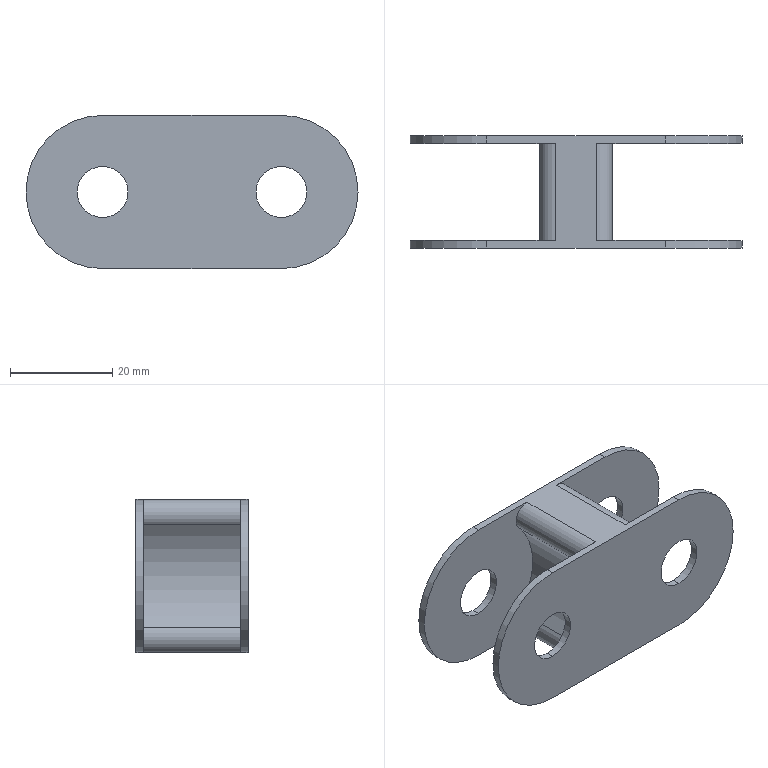Part | SolidWorks | features Extrusion 1, Fillet 1, ICE 1 | 1 solid | 26 faces | box 65 x 22 x 30 mm | volume 10120 mm3 | cylinder 18 | plane 8 | commonest cylinder face diameters 10 x8 30 x6 6 x4
STEP:
#1=CARTESIAN_POINT('',(-17.5,9.5,5.));
#2=VERTEX_POINT('',#1);
#3=CARTESIAN_POINT('',(-17.5,9.5,-5.));
#4=VERTEX_POINT('',#3);
#5=CARTESIAN_POINT('',(-17.5,9.5,0.));
#6=DIRECTION('',(0.,-1.,0.));
#7=DIRECTION('',(0.,0.,1.));
#8=AXIS2_PLACEMENT_3D('',#5,#6,#7);
#9=CIRCLE('',#8,5.);
#10=EDGE_CURVE('',#2,#4,#9,.T.);
#11=ORIENTED_EDGE('',*,*,#10,.T.);
#12=CARTESIAN_POINT('',(-17.5,11.,-5.));
#13=VERTEX_POINT('',#12);
#14=CARTESIAN_POINT('',(-17.5,-11.,-5.));
#15=DIRECTION('',(0.,1.,0.));
#16=VECTOR('',#15,1000.);
#17=LINE('',#14,#16);
#18=EDGE_CURVE('',#4,#13,#17,.T.);
#19=ORIENTED_EDGE('',*,*,#18,.T.);
#20=CARTESIAN_POINT('',(-17.5,11.,5.));
#21=VERTEX_POINT('',#20);
#22=CARTESIAN_POINT('',(-17.5,11.,0.));
#23=DIRECTION('',(0.,1.,0.));
#24=DIRECTION('',(0.,0.,1.));
#25=AXIS2_PLACEMENT_3D('',#22,#23,#24);
#26=CIRCLE('',#25,5.);
#27=EDGE_CURVE('',#13,#21,#26,.T.);
#28=ORIENTED_EDGE('',*,*,#27,.T.);
#29=CARTESIAN_POINT('',(-17.5,-11.,5.));
#30=DIRECTION('',(0.,1.,0.));
#31=VECTOR('',#30,1000.);
#32=LINE('',#29,#31);
#33=EDGE_CURVE('',#2,#21,#32,.T.);
#34=ORIENTED_EDGE('',*,*,#33,.F.);
#35=EDGE_LOOP('',(#11,#19,#28,#34));
#36=FACE_OUTER_BOUND('',#35,.T.);
#37=CARTESIAN_POINT('',(-17.5,-11.,0.));
#38=DIRECTION('',(0.,1.,0.));
#39=DIRECTION('',(0.,0.,1.));
#40=AXIS2_PLACEMENT_3D('',#37,#38,#39);
#41=CYLINDRICAL_SURFACE('',#40,5.);
#42=ADVANCED_FACE('',(#36),#41,.F.);
#43=CARTESIAN_POINT('',(17.5,9.5,5.));
#44=VERTEX_POINT('',#43);
#45=CARTESIAN_POINT('',(17.5,9.5,-5.));
#46=VERTEX_POINT('',#45);
#47=CARTESIAN_POINT('',(17.5,9.5,0.));
#48=DIRECTION('',(0.,-1.,0.));
#49=DIRECTION('',(0.,0.,1.));
#50=AXIS2_PLACEMENT_3D('',#47,#48,#49);
#51=CIRCLE('',#50,5.);
#52=EDGE_CURVE('',#44,#46,#51,.T.);
#53=ORIENTED_EDGE('',*,*,#52,.T.);
#54=CARTESIAN_POINT('',(17.5,11.,-5.));
#55=VERTEX_POINT('',#54);
#56=CARTESIAN_POINT('',(17.5,-11.,-5.));
#57=DIRECTION('',(0.,1.,0.));
#58=VECTOR('',#57,1000.);
#59=LINE('',#56,#58);
#60=EDGE_CURVE('',#46,#55,#59,.T.);
#61=ORIENTED_EDGE('',*,*,#60,.T.);
#62=CARTESIAN_POINT('',(17.5,11.,5.));
#63=VERTEX_POINT('',#62);
#64=CARTESIAN_POINT('',(17.5,11.,0.));
#65=DIRECTION('',(0.,1.,0.));
#66=DIRECTION('',(0.,0.,1.));
#67=AXIS2_PLACEMENT_3D('',#64,#65,#66);
#68=CIRCLE('',#67,5.);
#69=EDGE_CURVE('',#55,#63,#68,.T.);
#70=ORIENTED_EDGE('',*,*,#69,.T.);
#71=CARTESIAN_POINT('',(17.5,-11.,5.));
#72=DIRECTION('',(0.,1.,0.));
#73=VECTOR('',#72,1000.);
#74=LINE('',#71,#73);
#75=EDGE_CURVE('',#44,#63,#74,.T.);
#76=ORIENTED_EDGE('',*,*,#75,.F.);
#77=EDGE_LOOP('',(#53,#61,#70,#76));
#78=FACE_OUTER_BOUND('',#77,.T.);
#79=CARTESIAN_POINT('',(17.5,-11.,0.));
#80=DIRECTION('',(0.,1.,0.));
#81=DIRECTION('',(0.,0.,1.));
#82=AXIS2_PLACEMENT_3D('',#79,#80,#81);
#83=CYLINDRICAL_SURFACE('',#82,5.);
#84=ADVANCED_FACE('',(#78),#83,.F.);
#85=CARTESIAN_POINT('',(-17.5,-11.,-5.));
#86=VERTEX_POINT('',#85);
#87=CARTESIAN_POINT('',(-17.5,-11.,5.));
#88=VERTEX_POINT('',#87);
#89=CARTESIAN_POINT('',(-17.5,-11.,0.));
#90=DIRECTION('',(0.,1.,0.));
#91=DIRECTION('',(0.,0.,1.));
#92=AXIS2_PLACEMENT_3D('',#89,#90,#91);
#93=CIRCLE('',#92,5.);
#94=EDGE_CURVE('',#86,#88,#93,.T.);
#95=ORIENTED_EDGE('',*,*,#94,.F.);
#96=CARTESIAN_POINT('',(-17.5,-9.5,-5.));
#97=VERTEX_POINT('',#96);
#98=CARTESIAN_POINT('',(-17.5,-11.,-5.));
#99=DIRECTION('',(0.,1.,0.));
#100=VECTOR('',#99,1000.);
#101=LINE('',#98,#100);
#102=EDGE_CURVE('',#86,#97,#101,.T.);
#103=ORIENTED_EDGE('',*,*,#102,.T.);
#104=CARTESIAN_POINT('',(-17.5,-9.5,5.));
#105=VERTEX_POINT('',#104);
#106=CARTESIAN_POINT('',(-17.5,-9.5,0.));
#107=DIRECTION('',(0.,-1.,0.));
#108=DIRECTION('',(0.,0.,1.));
#109=AXIS2_PLACEMENT_3D('',#106,#107,#108);
#110=CIRCLE('',#109,5.);
#111=EDGE_CURVE('',#105,#97,#110,.T.);
#112=ORIENTED_EDGE('',*,*,#111,.F.);
#113=CARTESIAN_POINT('',(-17.5,-11.,5.));
#114=DIRECTION('',(0.,1.,0.));
#115=VECTOR('',#114,1000.);
#116=LINE('',#113,#115);
#117=EDGE_CURVE('',#88,#105,#116,.T.);
#118=ORIENTED_EDGE('',*,*,#117,.F.);
#119=EDGE_LOOP('',(#95,#103,#112,#118));
#120=FACE_OUTER_BOUND('',#119,.T.);
#121=CARTESIAN_POINT('',(-17.5,-11.,0.));
#122=DIRECTION('',(0.,1.,0.));
#123=DIRECTION('',(0.,0.,1.));
#124=AXIS2_PLACEMENT_3D('',#121,#122,#123);
#125=CYLINDRICAL_SURFACE('',#124,5.);
#126=ADVANCED_FACE('',(#120),#125,.F.);
#127=CARTESIAN_POINT('',(17.5,-11.,-5.));
#128=VERTEX_POINT('',#127);
#129=CARTESIAN_POINT('',(17.5,-11.,5.));
#130=VERTEX_POINT('',#129);
#131=CARTESIAN_POINT('',(17.5,-11.,0.));
#132=DIRECTION('',(0.,1.,0.));
#133=DIRECTION('',(0.,0.,1.));
#134=AXIS2_PLACEMENT_3D('',#131,#132,#133);
#135=CIRCLE('',#134,5.);
#136=EDGE_CURVE('',#128,#130,#135,.T.);
#137=ORIENTED_EDGE('',*,*,#136,.F.);
#138=CARTESIAN_POINT('',(17.5,-9.5,-5.));
#139=VERTEX_POINT('',#138);
#140=CARTESIAN_POINT('',(17.5,-11.,-5.));
#141=DIRECTION('',(0.,1.,0.));
#142=VECTOR('',#141,1000.);
#143=LINE('',#140,#142);
#144=EDGE_CURVE('',#128,#139,#143,.T.);
#145=ORIENTED_EDGE('',*,*,#144,.T.);
#146=CARTESIAN_POINT('',(17.5,-9.5,5.));
#147=VERTEX_POINT('',#146);
#148=CARTESIAN_POINT('',(17.5,-9.5,0.));
#149=DIRECTION('',(0.,-1.,0.));
#150=DIRECTION('',(0.,0.,1.));
#151=AXIS2_PLACEMENT_3D('',#148,#149,#150);
#152=CIRCLE('',#151,5.);
#153=EDGE_CURVE('',#147,#139,#152,.T.);
#154=ORIENTED_EDGE('',*,*,#153,.F.);
#155=CARTESIAN_POINT('',(17.5,-11.,5.));
#156=DIRECTION('',(0.,1.,0.));
#157=VECTOR('',#156,1000.);
#158=LINE('',#155,#157);
#159=EDGE_CURVE('',#130,#147,#158,.T.);
#160=ORIENTED_EDGE('',*,*,#159,.F.);
#161=EDGE_LOOP('',(#137,#145,#154,#160));
#162=FACE_OUTER_BOUND('',#161,.T.);
#163=CARTESIAN_POINT('',(17.5,-11.,0.));
#164=DIRECTION('',(0.,1.,0.));
#165=DIRECTION('',(0.,0.,1.));
#166=AXIS2_PLACEMENT_3D('',#163,#164,#165);
#167=CYLINDRICAL_SURFACE('',#166,5.);
#168=ADVANCED_FACE('',(#162),#167,.F.);
#169=CARTESIAN_POINT('',(17.5,-11.,-15.));
#170=VERTEX_POINT('',#169);
#171=CARTESIAN_POINT('',(17.5,-9.5,-15.));
#172=VERTEX_POINT('',#171);
#173=CARTESIAN_POINT('',(17.5,-11.,-15.));
#174=DIRECTION('',(0.,1.,0.));
#175=VECTOR('',#174,1000.);
#176=LINE('',#173,#175);
#177=EDGE_CURVE('',#170,#172,#176,.T.);
#178=ORIENTED_EDGE('',*,*,#177,.T.);
#179=CARTESIAN_POINT('',(17.5,-9.5,15.));
#180=VERTEX_POINT('',#179);
#181=CARTESIAN_POINT('',(17.5,-9.5,0.));
#182=DIRECTION('',(0.,1.,0.));
#183=DIRECTION('',(0.,0.,1.));
#184=AXIS2_PLACEMENT_3D('',#181,#182,#183);
#185=CIRCLE('',#184,15.);
#186=EDGE_CURVE('',#180,#172,#185,.T.);
#187=ORIENTED_EDGE('',*,*,#186,.F.);
#188=CARTESIAN_POINT('',(17.5,-11.,15.));
#189=VERTEX_POINT('',#188);
#190=CARTESIAN_POINT('',(17.5,-11.,15.));
#191=DIRECTION('',(0.,1.,0.));
#192=VECTOR('',#191,1000.);
#193=LINE('',#190,#192);
#194=EDGE_CURVE('',#189,#180,#193,.T.);
#195=ORIENTED_EDGE('',*,*,#194,.F.);
#196=CARTESIAN_POINT('',(17.5,-11.,0.));
#197=DIRECTION('',(0.,1.,0.));
#198=DIRECTION('',(0.,0.,1.));
#199=AXIS2_PLACEMENT_3D('',#196,#197,#198);
#200=CIRCLE('',#199,15.);
#201=EDGE_CURVE('',#189,#170,#200,.T.);
#202=ORIENTED_EDGE('',*,*,#201,.T.);
#203=EDGE_LOOP('',(#178,#187,#195,#202));
#204=FACE_OUTER_BOUND('',#203,.T.);
#205=CARTESIAN_POINT('',(17.5,-11.,0.));
#206=DIRECTION('',(0.,1.,0.));
#207=DIRECTION('',(0.,0.,1.));
#208=AXIS2_PLACEMENT_3D('',#205,#206,#207);
#209=CYLINDRICAL_SURFACE('',#208,15.);
#210=ADVANCED_FACE('',(#204),#209,.T.);
#211=ORIENTED_EDGE('',*,*,#144,.F.);
#212=CARTESIAN_POINT('',(17.5,-11.,0.));
#213=DIRECTION('',(0.,1.,0.));
#214=DIRECTION('',(0.,0.,1.));
#215=AXIS2_PLACEMENT_3D('',#212,#213,#214);
#216=CIRCLE('',#215,5.);
#217=EDGE_CURVE('',#130,#128,#216,.T.);
#218=ORIENTED_EDGE('',*,*,#217,.F.);
#219=ORIENTED_EDGE('',*,*,#159,.T.);
#220=CARTESIAN_POINT('',(17.5,-9.5,0.));
#221=DIRECTION('',(0.,-1.,0.));
#222=DIRECTION('',(0.,0.,1.));
#223=AXIS2_PLACEMENT_3D('',#220,#221,#222);
#224=CIRCLE('',#223,5.);
#225=EDGE_CURVE('',#139,#147,#224,.T.);
#226=ORIENTED_EDGE('',*,*,#225,.F.);
#227=EDGE_LOOP('',(#211,#218,#219,#226));
#228=FACE_OUTER_BOUND('',#227,.T.);
#229=CARTESIAN_POINT('',(17.5,-11.,0.));
#230=DIRECTION('',(0.,1.,0.));
#231=DIRECTION('',(0.,0.,1.));
#232=AXIS2_PLACEMENT_3D('',#229,#230,#231);
#233=CYLINDRICAL_SURFACE('',#232,5.);
#234=ADVANCED_FACE('',(#228),#233,.F.);
#235=CARTESIAN_POINT('',(-17.5,-11.,15.));
#236=VERTEX_POINT('',#235);
#237=CARTESIAN_POINT('',(-17.5,-9.5,15.));
#238=VERTEX_POINT('',#237);
#239=CARTESIAN_POINT('',(-17.5,-11.,15.));
#240=DIRECTION('',(0.,1.,0.));
#241=VECTOR('',#240,1000.);
#242=LINE('',#239,#241);
#243=EDGE_CURVE('',#236,#238,#242,.T.);
#244=ORIENTED_EDGE('',*,*,#243,.T.);
#245=CARTESIAN_POINT('',(-17.5,-9.5,-15.));
#246=VERTEX_POINT('',#245);
#247=CARTESIAN_POINT('',(-17.5,-9.5,0.));
#248=DIRECTION('',(0.,1.,0.));
#249=DIRECTION('',(0.,0.,1.));
#250=AXIS2_PLACEMENT_3D('',#247,#248,#249);
#251=CIRCLE('',#250,15.);
#252=EDGE_CURVE('',#246,#238,#251,.T.);
#253=ORIENTED_EDGE('',*,*,#252,.F.);
#254=CARTESIAN_POINT('',(-17.5,-11.,-15.));
#255=VERTEX_POINT('',#254);
#256=CARTESIAN_POINT('',(-17.5,-11.,-15.));
#257=DIRECTION('',(0.,1.,0.));
#258=VECTOR('',#257,1000.);
#259=LINE('',#256,#258);
#260=EDGE_CURVE('',#255,#246,#259,.T.);
#261=ORIENTED_EDGE('',*,*,#260,.F.);
#262=CARTESIAN_POINT('',(-17.5,-11.,0.));
#263=DIRECTION('',(0.,1.,0.));
#264=DIRECTION('',(0.,0.,1.));
#265=AXIS2_PLACEMENT_3D('',#262,#263,#264);
#266=CIRCLE('',#265,15.);
#267=EDGE_CURVE('',#255,#236,#266,.T.);
#268=ORIENTED_EDGE('',*,*,#267,.T.);
#269=EDGE_LOOP('',(#244,#253,#261,#268));
#270=FACE_OUTER_BOUND('',#269,.T.);
#271=CARTESIAN_POINT('',(-17.5,-11.,0.));
#272=DIRECTION('',(0.,1.,0.));
#273=DIRECTION('',(0.,0.,1.));
#274=AXIS2_PLACEMENT_3D('',#271,#272,#273);
#275=CYLINDRICAL_SURFACE('',#274,15.);
#276=ADVANCED_FACE('',(#270),#275,.T.);
#277=ORIENTED_EDGE('',*,*,#102,.F.);
#278=CARTESIAN_POINT('',(-17.5,-11.,0.));
#279=DIRECTION('',(0.,1.,0.));
#280=DIRECTION('',(0.,0.,1.));
#281=AXIS2_PLACEMENT_3D('',#278,#279,#280);
#282=CIRCLE('',#281,5.);
#283=EDGE_CURVE('',#88,#86,#282,.T.);
#284=ORIENTED_EDGE('',*,*,#283,.F.);
#285=ORIENTED_EDGE('',*,*,#117,.T.);
#286=CARTESIAN_POINT('',(-17.5,-9.5,0.));
#287=DIRECTION('',(0.,-1.,0.));
#288=DIRECTION('',(0.,0.,1.));
#289=AXIS2_PLACEMENT_3D('',#286,#287,#288);
#290=CIRCLE('',#289,5.);
#291=EDGE_CURVE('',#97,#105,#290,.T.);
#292=ORIENTED_EDGE('',*,*,#291,.F.);
#293=EDGE_LOOP('',(#277,#284,#285,#292));
#294=FACE_OUTER_BOUND('',#293,.T.);
#295=CARTESIAN_POINT('',(-17.5,-11.,0.));
#296=DIRECTION('',(0.,1.,0.));
#297=DIRECTION('',(0.,0.,1.));
#298=AXIS2_PLACEMENT_3D('',#295,#296,#297);
#299=CYLINDRICAL_SURFACE('',#298,5.);
#300=ADVANCED_FACE('',(#294),#299,.F.);
#301=CARTESIAN_POINT('',(-17.5,9.5,-15.));
#302=VERTEX_POINT('',#301);
#303=CARTESIAN_POINT('',(-17.5,9.5,15.));
#304=VERTEX_POINT('',#303);
#305=CARTESIAN_POINT('',(-17.5,9.5,0.));
#306=DIRECTION('',(0.,1.,0.));
#307=DIRECTION('',(0.,0.,1.));
#308=AXIS2_PLACEMENT_3D('',#305,#306,#307);
#309=CIRCLE('',#308,15.);
#310=EDGE_CURVE('',#302,#304,#309,.T.);
#311=ORIENTED_EDGE('',*,*,#310,.T.);
#312=CARTESIAN_POINT('',(-17.5,11.,15.));
#313=VERTEX_POINT('',#312);
#314=CARTESIAN_POINT('',(-17.5,-11.,15.));
#315=DIRECTION('',(0.,1.,0.));
#316=VECTOR('',#315,1000.);
#317=LINE('',#314,#316);
#318=EDGE_CURVE('',#304,#313,#317,.T.);
#319=ORIENTED_EDGE('',*,*,#318,.T.);
#320=CARTESIAN_POINT('',(-17.5,11.,-15.));
#321=VERTEX_POINT('',#320);
#322=CARTESIAN_POINT('',(-17.5,11.,0.));
#323=DIRECTION('',(0.,1.,0.));
#324=DIRECTION('',(0.,0.,1.));
#325=AXIS2_PLACEMENT_3D('',#322,#323,#324);
#326=CIRCLE('',#325,15.);
#327=EDGE_CURVE('',#321,#313,#326,.T.);
#328=ORIENTED_EDGE('',*,*,#327,.F.);
#329=CARTESIAN_POINT('',(-17.5,-11.,-15.));
#330=DIRECTION('',(0.,1.,0.));
#331=VECTOR('',#330,1000.);
#332=LINE('',#329,#331);
#333=EDGE_CURVE('',#302,#321,#332,.T.);
#334=ORIENTED_EDGE('',*,*,#333,.F.);
#335=EDGE_LOOP('',(#311,#319,#328,#334));
#336=FACE_OUTER_BOUND('',#335,.T.);
#337=CARTESIAN_POINT('',(-17.5,-11.,0.));
#338=DIRECTION('',(0.,1.,0.));
#339=DIRECTION('',(0.,0.,1.));
#340=AXIS2_PLACEMENT_3D('',#337,#338,#339);
#341=CYLINDRICAL_SURFACE('',#340,15.);
#342=ADVANCED_FACE('',(#336),#341,.T.);
#343=CARTESIAN_POINT('',(-4.084,-9.5,-15.));
#344=VERTEX_POINT('',#343);
#345=CARTESIAN_POINT('',(-4.084,9.5,-15.));
#346=VERTEX_POINT('',#345);
#347=CARTESIAN_POINT('',(-4.084,-11.,-15.));
#348=DIRECTION('',(0.,1.,0.));
#349=VECTOR('',#348,1000.);
#350=LINE('',#347,#349);
#351=EDGE_CURVE('',#344,#346,#350,.T.);
#352=ORIENTED_EDGE('',*,*,#351,.T.);
#353=CARTESIAN_POINT('',(-17.5,9.5,-15.));
#354=DIRECTION('',(-1.,0.,0.));
#355=VECTOR('',#354,1000.);
#356=LINE('',#353,#355);
#357=EDGE_CURVE('',#346,#302,#356,.T.);
#358=ORIENTED_EDGE('',*,*,#357,.T.);
#359=ORIENTED_EDGE('',*,*,#333,.T.);
#360=CARTESIAN_POINT('',(17.5,11.,-15.));
#361=VERTEX_POINT('',#360);
#362=CARTESIAN_POINT('',(-17.5,11.,-15.));
#363=DIRECTION('',(-1.,0.,0.));
#364=VECTOR('',#363,1000.);
#365=LINE('',#362,#364);
#366=EDGE_CURVE('',#361,#321,#365,.T.);
#367=ORIENTED_EDGE('',*,*,#366,.F.);
#368=CARTESIAN_POINT('',(17.5,9.5,-15.));
#369=VERTEX_POINT('',#368);
#370=CARTESIAN_POINT('',(17.5,-11.,-15.));
#371=DIRECTION('',(0.,1.,0.));
#372=VECTOR('',#371,1000.);
#373=LINE('',#370,#372);
#374=EDGE_CURVE('',#369,#361,#373,.T.);
#375=ORIENTED_EDGE('',*,*,#374,.F.);
#376=CARTESIAN_POINT('',(4.084,9.5,-15.));
#377=VERTEX_POINT('',#376);
#378=CARTESIAN_POINT('',(17.5,9.5,-15.));
#379=DIRECTION('',(-1.,0.,0.));
#380=VECTOR('',#379,1000.);
#381=LINE('',#378,#380);
#382=EDGE_CURVE('',#369,#377,#381,.T.);
#383=ORIENTED_EDGE('',*,*,#382,.T.);
#384=CARTESIAN_POINT('',(4.084,-9.5,-15.));
#385=VERTEX_POINT('',#384);
#386=CARTESIAN_POINT('',(4.084,-11.,-15.));
#387=DIRECTION('',(0.,-1.,0.));
#388=VECTOR('',#387,1000.);
#389=LINE('',#386,#388);
#390=EDGE_CURVE('',#377,#385,#389,.T.);
#391=ORIENTED_EDGE('',*,*,#390,.T.);
#392=CARTESIAN_POINT('',(-17.5,-9.5,-15.));
#393=DIRECTION('',(1.,0.,0.));
#394=VECTOR('',#393,1000.);
#395=LINE('',#392,#394);
#396=EDGE_CURVE('',#385,#172,#395,.T.);
#397=ORIENTED_EDGE('',*,*,#396,.T.);
#398=ORIENTED_EDGE('',*,*,#177,.F.);
#399=CARTESIAN_POINT('',(-17.5,-11.,-15.));
#400=DIRECTION('',(-1.,0.,0.));
#401=VECTOR('',#400,1000.);
#402=LINE('',#399,#401);
#403=EDGE_CURVE('',#170,#255,#402,.T.);
#404=ORIENTED_EDGE('',*,*,#403,.T.);
#405=ORIENTED_EDGE('',*,*,#260,.T.);
#406=CARTESIAN_POINT('',(-17.5,-9.5,-15.));
#407=DIRECTION('',(1.,0.,0.));
#408=VECTOR('',#407,1000.);
#409=LINE('',#406,#408);
#410=EDGE_CURVE('',#246,#344,#409,.T.);
#411=ORIENTED_EDGE('',*,*,#410,.T.);
#412=EDGE_LOOP('',(#352,#358,#359,#367,#375,#383,#391,#397,#398,#404,#405,#411));
#413=FACE_OUTER_BOUND('',#412,.T.);
#414=CARTESIAN_POINT('',(-17.5,-11.,-15.));
#415=DIRECTION('',(0.,0.,-1.));
#416=DIRECTION('',(-1.,0.,0.));
#417=AXIS2_PLACEMENT_3D('',#414,#415,#416);
#418=PLANE('',#417);
#419=ADVANCED_FACE('',(#413),#418,.T.);
#420=CARTESIAN_POINT('',(17.5,9.5,15.));
#421=VERTEX_POINT('',#420);
#422=CARTESIAN_POINT('',(17.5,9.5,0.));
#423=DIRECTION('',(0.,1.,0.));
#424=DIRECTION('',(0.,0.,1.));
#425=AXIS2_PLACEMENT_3D('',#422,#423,#424);
#426=CIRCLE('',#425,15.);
#427=EDGE_CURVE('',#421,#369,#426,.T.);
#428=ORIENTED_EDGE('',*,*,#427,.T.);
#429=ORIENTED_EDGE('',*,*,#374,.T.);
#430=CARTESIAN_POINT('',(17.5,11.,15.));
#431=VERTEX_POINT('',#430);
#432=CARTESIAN_POINT('',(17.5,11.,0.));
#433=DIRECTION('',(0.,1.,0.));
#434=DIRECTION('',(0.,0.,1.));
#435=AXIS2_PLACEMENT_3D('',#432,#433,#434);
#436=CIRCLE('',#435,15.);
#437=EDGE_CURVE('',#431,#361,#436,.T.);
#438=ORIENTED_EDGE('',*,*,#437,.F.);
#439=CARTESIAN_POINT('',(17.5,-11.,15.));
#440=DIRECTION('',(0.,1.,0.));
#441=VECTOR('',#440,1000.);
#442=LINE('',#439,#441);
#443=EDGE_CURVE('',#421,#431,#442,.T.);
#444=ORIENTED_EDGE('',*,*,#443,.F.);
#445=EDGE_LOOP('',(#428,#429,#438,#444));
#446=FACE_OUTER_BOUND('',#445,.T.);
#447=CARTESIAN_POINT('',(17.5,-11.,0.));
#448=DIRECTION('',(0.,1.,0.));
#449=DIRECTION('',(0.,0.,1.));
#450=AXIS2_PLACEMENT_3D('',#447,#448,#449);
#451=CYLINDRICAL_SURFACE('',#450,15.);
#452=ADVANCED_FACE('',(#446),#451,.T.);
#453=CARTESIAN_POINT('',(4.084,-9.5,15.));
#454=VERTEX_POINT('',#453);
#455=CARTESIAN_POINT('',(4.084,9.5,15.));
#456=VERTEX_POINT('',#455);
#457=CARTESIAN_POINT('',(4.084,-11.,15.));
#458=DIRECTION('',(0.,1.,0.));
#459=VECTOR('',#458,1000.);
#460=LINE('',#457,#459);
#461=EDGE_CURVE('',#454,#456,#460,.T.);
#462=ORIENTED_EDGE('',*,*,#461,.T.);
#463=CARTESIAN_POINT('',(17.5,9.5,15.));
#464=DIRECTION('',(1.,0.,0.));
#465=VECTOR('',#464,1000.);
#466=LINE('',#463,#465);
#467=EDGE_CURVE('',#456,#421,#466,.T.);
#468=ORIENTED_EDGE('',*,*,#467,.T.);
#469=ORIENTED_EDGE('',*,*,#443,.T.);
#470=CARTESIAN_POINT('',(-17.5,11.,15.));
#471=DIRECTION('',(1.,0.,0.));
#472=VECTOR('',#471,1000.);
#473=LINE('',#470,#472);
#474=EDGE_CURVE('',#313,#431,#473,.T.);
#475=ORIENTED_EDGE('',*,*,#474,.F.);
#476=ORIENTED_EDGE('',*,*,#318,.F.);
#477=CARTESIAN_POINT('',(-4.084,9.5,15.));
#478=VERTEX_POINT('',#477);
#479=CARTESIAN_POINT('',(-17.5,9.5,15.));
#480=DIRECTION('',(1.,0.,0.));
#481=VECTOR('',#480,1000.);
#482=LINE('',#479,#481);
#483=EDGE_CURVE('',#304,#478,#482,.T.);
#484=ORIENTED_EDGE('',*,*,#483,.T.);
#485=CARTESIAN_POINT('',(-4.084,-9.5,15.));
#486=VERTEX_POINT('',#485);
#487=CARTESIAN_POINT('',(-4.084,-11.,15.));
#488=DIRECTION('',(0.,-1.,0.));
#489=VECTOR('',#488,1000.);
#490=LINE('',#487,#489);
#491=EDGE_CURVE('',#478,#486,#490,.T.);
#492=ORIENTED_EDGE('',*,*,#491,.T.);
#493=CARTESIAN_POINT('',(-17.5,-9.5,15.));
#494=DIRECTION('',(-1.,0.,0.));
#495=VECTOR('',#494,1000.);
#496=LINE('',#493,#495);
#497=EDGE_CURVE('',#486,#238,#496,.T.);
#498=ORIENTED_EDGE('',*,*,#497,.T.);
#499=ORIENTED_EDGE('',*,*,#243,.F.);
#500=CARTESIAN_POINT('',(-17.5,-11.,15.));
#501=DIRECTION('',(1.,0.,0.));
#502=VECTOR('',#501,1000.);
#503=LINE('',#500,#502);
#504=EDGE_CURVE('',#236,#189,#503,.T.);
#505=ORIENTED_EDGE('',*,*,#504,.T.);
#506=ORIENTED_EDGE('',*,*,#194,.T.);
#507=CARTESIAN_POINT('',(-17.5,-9.5,15.));
#508=DIRECTION('',(-1.,0.,0.));
#509=VECTOR('',#508,1000.);
#510=LINE('',#507,#509);
#511=EDGE_CURVE('',#180,#454,#510,.T.);
#512=ORIENTED_EDGE('',*,*,#511,.T.);
#513=EDGE_LOOP('',(#462,#468,#469,#475,#476,#484,#492,#498,#499,#505,#506,#512));
#514=FACE_OUTER_BOUND('',#513,.T.);
#515=CARTESIAN_POINT('',(-17.5,-11.,15.));
#516=DIRECTION('',(0.,0.,1.));
#517=DIRECTION('',(1.,0.,0.));
#518=AXIS2_PLACEMENT_3D('',#515,#516,#517);
#519=PLANE('',#518);
#520=ADVANCED_FACE('',(#514),#519,.T.);
#521=ORIENTED_EDGE('',*,*,#283,.T.);
#522=ORIENTED_EDGE('',*,*,#94,.T.);
#523=EDGE_LOOP('',(#521,#522));
#524=FACE_BOUND('',#523,.T.);
#525=ORIENTED_EDGE('',*,*,#217,.T.);
#526=ORIENTED_EDGE('',*,*,#136,.T.);
#527=EDGE_LOOP('',(#525,#526));
#528=FACE_BOUND('',#527,.T.);
#529=ORIENTED_EDGE('',*,*,#267,.F.);
#530=ORIENTED_EDGE('',*,*,#403,.F.);
#531=ORIENTED_EDGE('',*,*,#201,.F.);
#532=ORIENTED_EDGE('',*,*,#504,.F.);
#533=EDGE_LOOP('',(#529,#530,#531,#532));
#534=FACE_OUTER_BOUND('',#533,.T.);
#535=CARTESIAN_POINT('',(-17.5,-11.,0.));
#536=DIRECTION('',(0.,1.,0.));
#537=DIRECTION('',(0.,0.,1.));
#538=AXIS2_PLACEMENT_3D('',#535,#536,#537);
#539=PLANE('',#538);
#540=ADVANCED_FACE('',(#524,#528,#534),#539,.F.);
#541=ORIENTED_EDGE('',*,*,#60,.F.);
#542=CARTESIAN_POINT('',(17.5,9.5,0.));
#543=DIRECTION('',(0.,-1.,0.));
#544=DIRECTION('',(0.,0.,1.));
#545=AXIS2_PLACEMENT_3D('',#542,#543,#544);
#546=CIRCLE('',#545,5.);
#547=EDGE_CURVE('',#46,#44,#546,.T.);
#548=ORIENTED_EDGE('',*,*,#547,.T.);
#549=ORIENTED_EDGE('',*,*,#75,.T.);
#550=CARTESIAN_POINT('',(17.5,11.,0.));
#551=DIRECTION('',(0.,1.,0.));
#552=DIRECTION('',(0.,0.,1.));
#553=AXIS2_PLACEMENT_3D('',#550,#551,#552);
#554=CIRCLE('',#553,5.);
#555=EDGE_CURVE('',#63,#55,#554,.T.);
#556=ORIENTED_EDGE('',*,*,#555,.T.);
#557=EDGE_LOOP('',(#541,#548,#549,#556));
#558=FACE_OUTER_BOUND('',#557,.T.);
#559=CARTESIAN_POINT('',(17.5,-11.,0.));
#560=DIRECTION('',(0.,1.,0.));
#561=DIRECTION('',(0.,0.,1.));
#562=AXIS2_PLACEMENT_3D('',#559,#560,#561);
#563=CYLINDRICAL_SURFACE('',#562,5.);
#564=ADVANCED_FACE('',(#558),#563,.F.);
#565=ORIENTED_EDGE('',*,*,#18,.F.);
#566=CARTESIAN_POINT('',(-17.5,9.5,0.));
#567=DIRECTION('',(0.,-1.,0.));
#568=DIRECTION('',(0.,0.,1.));
#569=AXIS2_PLACEMENT_3D('',#566,#567,#568);
#570=CIRCLE('',#569,5.);
#571=EDGE_CURVE('',#4,#2,#570,.T.);
#572=ORIENTED_EDGE('',*,*,#571,.T.);
#573=ORIENTED_EDGE('',*,*,#33,.T.);
#574=CARTESIAN_POINT('',(-17.5,11.,0.));
#575=DIRECTION('',(0.,1.,0.));
#576=DIRECTION('',(0.,0.,1.));
#577=AXIS2_PLACEMENT_3D('',#574,#575,#576);
#578=CIRCLE('',#577,5.);
#579=EDGE_CURVE('',#21,#13,#578,.T.);
#580=ORIENTED_EDGE('',*,*,#579,.T.);
#581=EDGE_LOOP('',(#565,#572,#573,#580));
#582=FACE_OUTER_BOUND('',#581,.T.);
#583=CARTESIAN_POINT('',(-17.5,-11.,0.));
#584=DIRECTION('',(0.,1.,0.));
#585=DIRECTION('',(0.,0.,1.));
#586=AXIS2_PLACEMENT_3D('',#583,#584,#585);
#587=CYLINDRICAL_SURFACE('',#586,5.);
#588=ADVANCED_FACE('',(#582),#587,.F.);
#589=ORIENTED_EDGE('',*,*,#555,.F.);
#590=ORIENTED_EDGE('',*,*,#69,.F.);
#591=EDGE_LOOP('',(#589,#590));
#592=FACE_BOUND('',#591,.T.);
#593=ORIENTED_EDGE('',*,*,#327,.T.);
#594=ORIENTED_EDGE('',*,*,#474,.T.);
#595=ORIENTED_EDGE('',*,*,#437,.T.);
#596=ORIENTED_EDGE('',*,*,#366,.T.);
#597=EDGE_LOOP('',(#593,#594,#595,#596));
#598=FACE_OUTER_BOUND('',#597,.T.);
#599=ORIENTED_EDGE('',*,*,#579,.F.);
#600=ORIENTED_EDGE('',*,*,#27,.F.);
#601=EDGE_LOOP('',(#599,#600));
#602=FACE_BOUND('',#601,.T.);
#603=CARTESIAN_POINT('',(-17.5,11.,0.));
#604=DIRECTION('',(0.,1.,0.));
#605=DIRECTION('',(0.,0.,1.));
#606=AXIS2_PLACEMENT_3D('',#603,#604,#605);
#607=PLANE('',#606);
#608=ADVANCED_FACE('',(#592,#598,#602),#607,.T.);
#609=CARTESIAN_POINT('',(-6.32,9.5,10.));
#610=VERTEX_POINT('',#609);
#611=CARTESIAN_POINT('',(-6.32,9.5,-10.));
#612=VERTEX_POINT('',#611);
#613=CARTESIAN_POINT('',(-17.5,9.5,0.));
#614=DIRECTION('',(0.,1.,0.));
#615=DIRECTION('',(0.,0.,1.));
#616=AXIS2_PLACEMENT_3D('',#613,#614,#615);
#617=CIRCLE('',#616,15.);
#618=EDGE_CURVE('',#610,#612,#617,.T.);
#619=ORIENTED_EDGE('',*,*,#618,.F.);
#620=CARTESIAN_POINT('',(-4.084,9.5,12.));
#621=DIRECTION('',(0.,1.,0.));
#622=DIRECTION('',(0.,0.,1.));
#623=AXIS2_PLACEMENT_3D('',#620,#621,#622);
#624=CIRCLE('',#623,3.);
#625=EDGE_CURVE('',#610,#478,#624,.T.);
#626=ORIENTED_EDGE('',*,*,#625,.T.);
#627=ORIENTED_EDGE('',*,*,#483,.F.);
#628=ORIENTED_EDGE('',*,*,#310,.F.);
#629=ORIENTED_EDGE('',*,*,#357,.F.);
#630=CARTESIAN_POINT('',(-4.084,9.5,-12.));
#631=DIRECTION('',(0.,1.,0.));
#632=DIRECTION('',(0.,0.,1.));
#633=AXIS2_PLACEMENT_3D('',#630,#631,#632);
#634=CIRCLE('',#633,3.);
#635=EDGE_CURVE('',#346,#612,#634,.T.);
#636=ORIENTED_EDGE('',*,*,#635,.T.);
#637=EDGE_LOOP('',(#619,#626,#627,#628,#629,#636));
#638=FACE_OUTER_BOUND('',#637,.T.);
#639=ORIENTED_EDGE('',*,*,#10,.F.);
#640=ORIENTED_EDGE('',*,*,#571,.F.);
#641=EDGE_LOOP('',(#639,#640));
#642=FACE_BOUND('',#641,.T.);
#643=CARTESIAN_POINT('',(-17.5,9.5,0.));
#644=DIRECTION('',(0.,1.,0.));
#645=DIRECTION('',(0.,0.,1.));
#646=AXIS2_PLACEMENT_3D('',#643,#644,#645);
#647=PLANE('',#646);
#648=ADVANCED_FACE('',(#638,#642),#647,.F.);
#649=ORIENTED_EDGE('',*,*,#252,.T.);
#650=ORIENTED_EDGE('',*,*,#497,.F.);
#651=CARTESIAN_POINT('',(-6.32,-9.5,10.));
#652=VERTEX_POINT('',#651);
#653=CARTESIAN_POINT('',(-4.084,-9.5,12.));
#654=DIRECTION('',(0.,-1.,0.));
#655=DIRECTION('',(0.,0.,1.));
#656=AXIS2_PLACEMENT_3D('',#653,#654,#655);
#657=CIRCLE('',#656,3.);
#658=EDGE_CURVE('',#486,#652,#657,.T.);
#659=ORIENTED_EDGE('',*,*,#658,.T.);
#660=CARTESIAN_POINT('',(-6.32,-9.5,-10.));
#661=VERTEX_POINT('',#660);
#662=CARTESIAN_POINT('',(-17.5,-9.5,0.));
#663=DIRECTION('',(0.,1.,0.));
#664=DIRECTION('',(0.,0.,1.));
#665=AXIS2_PLACEMENT_3D('',#662,#663,#664);
#666=CIRCLE('',#665,15.);
#667=EDGE_CURVE('',#652,#661,#666,.T.);
#668=ORIENTED_EDGE('',*,*,#667,.T.);
#669=CARTESIAN_POINT('',(-4.084,-9.5,-12.));
#670=DIRECTION('',(0.,-1.,0.));
#671=DIRECTION('',(0.,0.,1.));
#672=AXIS2_PLACEMENT_3D('',#669,#670,#671);
#673=CIRCLE('',#672,3.);
#674=EDGE_CURVE('',#661,#344,#673,.T.);
#675=ORIENTED_EDGE('',*,*,#674,.T.);
#676=ORIENTED_EDGE('',*,*,#410,.F.);
#677=EDGE_LOOP('',(#649,#650,#659,#668,#675,#676));
#678=FACE_OUTER_BOUND('',#677,.T.);
#679=ORIENTED_EDGE('',*,*,#111,.T.);
#680=ORIENTED_EDGE('',*,*,#291,.T.);
#681=EDGE_LOOP('',(#679,#680));
#682=FACE_BOUND('',#681,.T.);
#683=CARTESIAN_POINT('',(-17.5,-9.5,0.));
#684=DIRECTION('',(0.,1.,0.));
#685=DIRECTION('',(0.,0.,1.));
#686=AXIS2_PLACEMENT_3D('',#683,#684,#685);
#687=PLANE('',#686);
#688=ADVANCED_FACE('',(#678,#682),#687,.T.);
#689=ORIENTED_EDGE('',*,*,#618,.T.);
#690=CARTESIAN_POINT('',(-6.32,9.5,-10.));
#691=DIRECTION('',(0.,-1.,0.));
#692=VECTOR('',#691,1000.);
#693=LINE('',#690,#692);
#694=EDGE_CURVE('',#612,#661,#693,.T.);
#695=ORIENTED_EDGE('',*,*,#694,.T.);
#696=ORIENTED_EDGE('',*,*,#667,.F.);
#697=CARTESIAN_POINT('',(-6.32,9.5,10.));
#698=DIRECTION('',(0.,1.,0.));
#699=VECTOR('',#698,1000.);
#700=LINE('',#697,#699);
#701=EDGE_CURVE('',#652,#610,#700,.T.);
#702=ORIENTED_EDGE('',*,*,#701,.T.);
#703=EDGE_LOOP('',(#689,#695,#696,#702));
#704=FACE_OUTER_BOUND('',#703,.T.);
#705=CARTESIAN_POINT('',(-17.5,9.5,0.));
#706=DIRECTION('',(0.,-1.,0.));
#707=DIRECTION('',(0.,0.,-1.));
#708=AXIS2_PLACEMENT_3D('',#705,#706,#707);
#709=CYLINDRICAL_SURFACE('',#708,15.);
#710=ADVANCED_FACE('',(#704),#709,.F.);
#711=CARTESIAN_POINT('',(6.32,-9.5,-10.));
#712=VERTEX_POINT('',#711);
#713=CARTESIAN_POINT('',(6.32,-9.5,10.));
#714=VERTEX_POINT('',#713);
#715=CARTESIAN_POINT('',(17.5,-9.5,0.));
#716=DIRECTION('',(0.,1.,0.));
#717=DIRECTION('',(0.,0.,1.));
#718=AXIS2_PLACEMENT_3D('',#715,#716,#717);
#719=CIRCLE('',#718,15.);
#720=EDGE_CURVE('',#712,#714,#719,.T.);
#721=ORIENTED_EDGE('',*,*,#720,.F.);
#722=CARTESIAN_POINT('',(6.32,9.5,-10.));
#723=VERTEX_POINT('',#722);
#724=CARTESIAN_POINT('',(6.32,9.5,-10.));
#725=DIRECTION('',(0.,1.,0.));
#726=VECTOR('',#725,1000.);
#727=LINE('',#724,#726);
#728=EDGE_CURVE('',#712,#723,#727,.T.);
#729=ORIENTED_EDGE('',*,*,#728,.T.);
#730=CARTESIAN_POINT('',(6.32,9.5,10.));
#731=VERTEX_POINT('',#730);
#732=CARTESIAN_POINT('',(17.5,9.5,0.));
#733=DIRECTION('',(0.,1.,0.));
#734=DIRECTION('',(0.,0.,1.));
#735=AXIS2_PLACEMENT_3D('',#732,#733,#734);
#736=CIRCLE('',#735,15.);
#737=EDGE_CURVE('',#723,#731,#736,.T.);
#738=ORIENTED_EDGE('',*,*,#737,.T.);
#739=CARTESIAN_POINT('',(6.32,9.5,10.));
#740=DIRECTION('',(0.,-1.,0.));
#741=VECTOR('',#740,1000.);
#742=LINE('',#739,#741);
#743=EDGE_CURVE('',#731,#714,#742,.T.);
#744=ORIENTED_EDGE('',*,*,#743,.T.);
#745=EDGE_LOOP('',(#721,#729,#738,#744));
#746=FACE_OUTER_BOUND('',#745,.T.);
#747=CARTESIAN_POINT('',(17.5,9.5,0.));
#748=DIRECTION('',(0.,-1.,0.));
#749=DIRECTION('',(0.,0.,-1.));
#750=AXIS2_PLACEMENT_3D('',#747,#748,#749);
#751=CYLINDRICAL_SURFACE('',#750,15.);
#752=ADVANCED_FACE('',(#746),#751,.F.);
#753=ORIENTED_EDGE('',*,*,#427,.F.);
#754=ORIENTED_EDGE('',*,*,#467,.F.);
#755=CARTESIAN_POINT('',(4.084,9.5,12.));
#756=DIRECTION('',(0.,1.,0.));
#757=DIRECTION('',(0.,0.,1.));
#758=AXIS2_PLACEMENT_3D('',#755,#756,#757);
#759=CIRCLE('',#758,3.);
#760=EDGE_CURVE('',#456,#731,#759,.T.);
#761=ORIENTED_EDGE('',*,*,#760,.T.);
#762=ORIENTED_EDGE('',*,*,#737,.F.);
#763=CARTESIAN_POINT('',(4.084,9.5,-12.));
#764=DIRECTION('',(0.,1.,0.));
#765=DIRECTION('',(0.,0.,1.));
#766=AXIS2_PLACEMENT_3D('',#763,#764,#765);
#767=CIRCLE('',#766,3.);
#768=EDGE_CURVE('',#723,#377,#767,.T.);
#769=ORIENTED_EDGE('',*,*,#768,.T.);
#770=ORIENTED_EDGE('',*,*,#382,.F.);
#771=EDGE_LOOP('',(#753,#754,#761,#762,#769,#770));
#772=FACE_OUTER_BOUND('',#771,.T.);
#773=ORIENTED_EDGE('',*,*,#52,.F.);
#774=ORIENTED_EDGE('',*,*,#547,.F.);
#775=EDGE_LOOP('',(#773,#774));
#776=FACE_BOUND('',#775,.T.);
#777=CARTESIAN_POINT('',(17.5,9.5,0.));
#778=DIRECTION('',(0.,1.,0.));
#779=DIRECTION('',(0.,0.,1.));
#780=AXIS2_PLACEMENT_3D('',#777,#778,#779);
#781=PLANE('',#780);
#782=ADVANCED_FACE('',(#772,#776),#781,.F.);
#783=ORIENTED_EDGE('',*,*,#186,.T.);
#784=ORIENTED_EDGE('',*,*,#396,.F.);
#785=CARTESIAN_POINT('',(4.084,-9.5,-12.));
#786=DIRECTION('',(0.,-1.,0.));
#787=DIRECTION('',(0.,0.,1.));
#788=AXIS2_PLACEMENT_3D('',#785,#786,#787);
#789=CIRCLE('',#788,3.);
#790=EDGE_CURVE('',#385,#712,#789,.T.);
#791=ORIENTED_EDGE('',*,*,#790,.T.);
#792=ORIENTED_EDGE('',*,*,#720,.T.);
#793=CARTESIAN_POINT('',(4.084,-9.5,12.));
#794=DIRECTION('',(0.,-1.,0.));
#795=DIRECTION('',(0.,0.,1.));
#796=AXIS2_PLACEMENT_3D('',#793,#794,#795);
#797=CIRCLE('',#796,3.);
#798=EDGE_CURVE('',#714,#454,#797,.T.);
#799=ORIENTED_EDGE('',*,*,#798,.T.);
#800=ORIENTED_EDGE('',*,*,#511,.F.);
#801=EDGE_LOOP('',(#783,#784,#791,#792,#799,#800));
#802=FACE_OUTER_BOUND('',#801,.T.);
#803=ORIENTED_EDGE('',*,*,#153,.T.);
#804=ORIENTED_EDGE('',*,*,#225,.T.);
#805=EDGE_LOOP('',(#803,#804));
#806=FACE_BOUND('',#805,.T.);
#807=CARTESIAN_POINT('',(17.5,-9.5,0.));
#808=DIRECTION('',(0.,1.,0.));
#809=DIRECTION('',(0.,0.,1.));
#810=AXIS2_PLACEMENT_3D('',#807,#808,#809);
#811=PLANE('',#810);
#812=ADVANCED_FACE('',(#802,#806),#811,.T.);
#813=ORIENTED_EDGE('',*,*,#674,.F.);
#814=ORIENTED_EDGE('',*,*,#694,.F.);
#815=ORIENTED_EDGE('',*,*,#635,.F.);
#816=ORIENTED_EDGE('',*,*,#351,.F.);
#817=EDGE_LOOP('',(#813,#814,#815,#816));
#818=FACE_OUTER_BOUND('',#817,.T.);
#819=CARTESIAN_POINT('',(-4.084,9.5,-12.));
#820=DIRECTION('',(0.,-1.,0.));
#821=DIRECTION('',(0.,0.,-1.));
#822=AXIS2_PLACEMENT_3D('',#819,#820,#821);
#823=CYLINDRICAL_SURFACE('',#822,3.);
#824=ADVANCED_FACE('',(#818),#823,.T.);
#825=ORIENTED_EDGE('',*,*,#790,.F.);
#826=ORIENTED_EDGE('',*,*,#390,.F.);
#827=ORIENTED_EDGE('',*,*,#768,.F.);
#828=ORIENTED_EDGE('',*,*,#728,.F.);
#829=EDGE_LOOP('',(#825,#826,#827,#828));
#830=FACE_OUTER_BOUND('',#829,.T.);
#831=CARTESIAN_POINT('',(4.084,9.5,-12.));
#832=DIRECTION('',(0.,-1.,0.));
#833=DIRECTION('',(0.,0.,-1.));
#834=AXIS2_PLACEMENT_3D('',#831,#832,#833);
#835=CYLINDRICAL_SURFACE('',#834,3.);
#836=ADVANCED_FACE('',(#830),#835,.T.);
#837=ORIENTED_EDGE('',*,*,#798,.F.);
#838=ORIENTED_EDGE('',*,*,#743,.F.);
#839=ORIENTED_EDGE('',*,*,#760,.F.);
#840=ORIENTED_EDGE('',*,*,#461,.F.);
#841=EDGE_LOOP('',(#837,#838,#839,#840));
#842=FACE_OUTER_BOUND('',#841,.T.);
#843=CARTESIAN_POINT('',(4.084,9.5,12.));
#844=DIRECTION('',(0.,-1.,0.));
#845=DIRECTION('',(0.,0.,-1.));
#846=AXIS2_PLACEMENT_3D('',#843,#844,#845);
#847=CYLINDRICAL_SURFACE('',#846,3.);
#848=ADVANCED_FACE('',(#842),#847,.T.);
#849=ORIENTED_EDGE('',*,*,#658,.F.);
#850=ORIENTED_EDGE('',*,*,#491,.F.);
#851=ORIENTED_EDGE('',*,*,#625,.F.);
#852=ORIENTED_EDGE('',*,*,#701,.F.);
#853=EDGE_LOOP('',(#849,#850,#851,#852));
#854=FACE_OUTER_BOUND('',#853,.T.);
#855=CARTESIAN_POINT('',(-4.084,9.5,12.));
#856=DIRECTION('',(0.,-1.,0.));
#857=DIRECTION('',(0.,0.,-1.));
#858=AXIS2_PLACEMENT_3D('',#855,#856,#857);
#859=CYLINDRICAL_SURFACE('',#858,3.);
#860=ADVANCED_FACE('',(#854),#859,.T.);
#861=CLOSED_SHELL('',(#42,#84,#126,#168,#210,#234,#276,#300,#342,#419,#452,#520,#540,#564,#588,#608,#648,#688,#710,#752,#782,#812,#824,#836,#848,#860));
#862=MANIFOLD_SOLID_BREP('',#861);
#863=CARTESIAN_POINT('',(0.,0.,0.));
#864=DIRECTION('',(0.,0.,1.));
#865=DIRECTION('',(1.,0.,0.));
#866=AXIS2_PLACEMENT_3D('',#863,#864,#865);
#867=(LENGTH_UNIT()NAMED_UNIT(*)SI_UNIT(.MILLI.,.METRE.));
#868=UNCERTAINTY_MEASURE_WITH_UNIT(LENGTH_MEASURE(0.00001),#867,'','');
#869=(NAMED_UNIT(*)PLANE_ANGLE_UNIT()SI_UNIT($,.RADIAN.));
#870=(NAMED_UNIT(*)SI_UNIT($,.STERADIAN.)SOLID_ANGLE_UNIT());
#871=(GEOMETRIC_REPRESENTATION_CONTEXT(3)GLOBAL_UNCERTAINTY_ASSIGNED_CONTEXT((#868))GLOBAL_UNIT_ASSIGNED_CONTEXT((#867,#869,#870))REPRESENTATION_CONTEXT('',''));
#872=ADVANCED_BREP_SHAPE_REPRESENTATION('',(#862,#866),#871);